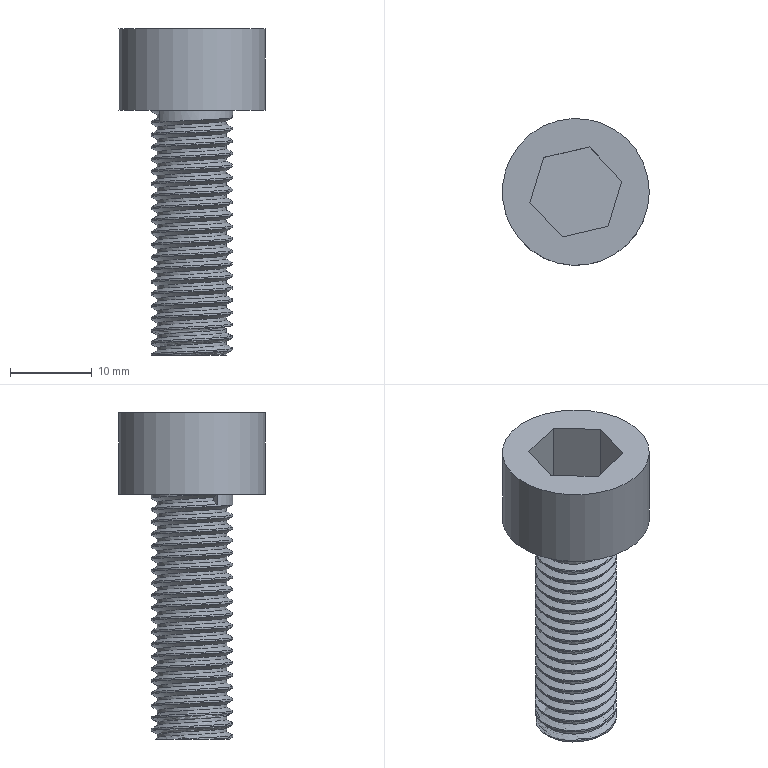Part | NX | features DATUM_CSYS 4, EXTRUDE 3, SKETCH 3, THREADS 1 | 1 solid | 17 faces | box 18 x 18 x 40 mm | volume 3838 mm3 | plane 11 | cylinder 3 | spline 3 | commonest cylinder face diameters 8.5 x1 10 x1 18 x1